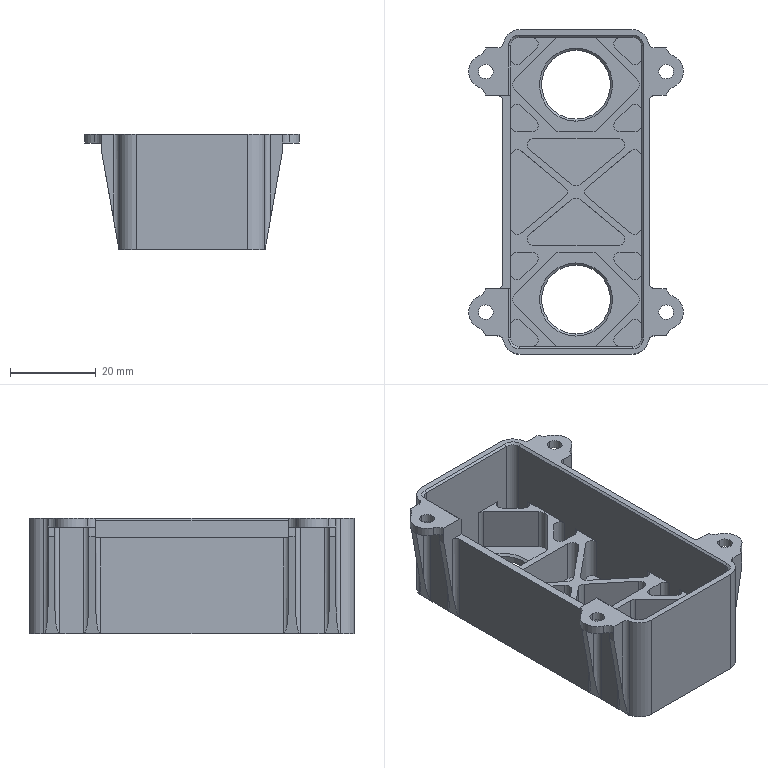NC program | NX | posted with a generic post | part box 50 x 75.58 x 26.8 mm
Lines 15469 to 16372 of 35818:
(CAVITY_MILL_COPY_COPY_COPY , TOOL : D3)
N30900 T17 M6
N30902 G54
N30904 G17 G0 G90 X-12.674 Y-33.89 S8500 M3
N30906 G43 Z30. H17
N30908 Z-13.949
N30910 G94 G1 Z-14.949 F1000.
N30912 X-12.616 Y-33.99
N30914 G3 X-11.75 Y-34.49 R1.
N30916 G1 X-10.295 F800.
N30918 X-11.324 Y-33.461
N30920 G3 X-12.29 Y-33.202 R1.
N30922 G1 X-12.401 Y-33.232
N30924 Z-13.949
N30926 G0 X-12.674 Y-33.89 Z-14.099
N30928 G1 Z-15.099 F1000.
N30930 X-12.616 Y-33.99
N30932 G3 X-11.75 Y-34.49 R1.
N30934 G1 X-10.295 F800.
N30936 X-11.324 Y-33.461
N30938 G3 X-12.29 Y-33.202 R1.
N30940 G1 X-12.401 Y-33.232
N30942 Z-14.099
N30944 G0 X-12.674 Y-33.89 Z-14.248
N30946 G1 Z-15.248 F1000.
N30948 X-12.616 Y-33.99
N30950 G3 X-11.75 Y-34.49 R1.
N30952 G1 X-10.295 F800.
N30954 X-11.324 Y-33.461
N30956 G3 X-12.29 Y-33.202 R1.
N30958 G1 X-12.401 Y-33.232
N30960 Z-14.248
N30962 G0 X-12.674 Y-33.89 Z-14.397
N30964 G1 Z-15.397 F1000.
N30966 X-12.616 Y-33.99
N30968 G3 X-11.75 Y-34.49 R1.
N30970 G1 X-10.295 F800.
N30972 X-11.324 Y-33.461
N30974 G3 X-12.29 Y-33.202 R1.
N30976 G1 X-12.401 Y-33.232
N30978 Z-14.397
N30980 G0 X-12.674 Y-33.89 Z-14.546
N30982 G1 Z-15.546 F1000.
N30984 X-12.616 Y-33.99
N30986 G3 X-11.75 Y-34.49 R1.
N30988 G1 X-10.295 F800.
N30990 X-11.324 Y-33.461
N30992 G3 X-12.29 Y-33.202 R1.
N30994 G1 X-12.401 Y-33.232
N30996 Z-14.546
N30998 G0 X-12.674 Y-33.89 Z-14.696
N31000 G1 Z-15.696 F1000.
N31002 X-12.616 Y-33.99
N31004 G3 X-11.75 Y-34.49 R1.
N31006 G1 X-10.295 F800.
N31008 X-11.324 Y-33.461
N31010 G3 X-12.29 Y-33.202 R1.
N31012 G1 X-12.401 Y-33.232
N31014 Z-14.696
N31016 G0 X-12.674 Y-33.89 Z-14.845
N31018 G1 Z-15.845 F1000.
N31020 X-12.616 Y-33.99
N31022 G3 X-11.75 Y-34.49 R1.
N31024 G1 X-10.295 F800.
N31026 X-11.324 Y-33.461
N31028 G3 X-12.29 Y-33.202 R1.
N31030 G1 X-12.401 Y-33.232
N31032 Z-14.845
N31034 G0 X-12.674 Y-33.89 Z-14.994
N31036 G1 Z-15.994 F1000.
N31038 X-12.616 Y-33.99
N31040 G3 X-11.75 Y-34.49 R1.
N31042 G1 X-10.295 F800.
N31044 X-11.324 Y-33.461
N31046 G3 X-12.29 Y-33.202 R1.
N31048 G1 X-12.401 Y-33.232
N31050 Z-14.994
N31052 G0 X-12.674 Y-33.89 Z-15.143
N31054 G1 Z-16.143 F1000.
N31056 X-12.616 Y-33.99
N31058 G3 X-11.75 Y-34.49 R1.
N31060 G1 X-10.295 F800.
N31062 X-11.324 Y-33.461
N31064 G3 X-12.29 Y-33.202 R1.
N31066 G1 X-12.401 Y-33.232
N31068 Z-15.143
N31070 G0 X-12.674 Y-33.89 Z-15.293
N31072 G1 Z-16.293 F1000.
N31074 X-12.616 Y-33.99
N31076 G3 X-11.75 Y-34.49 R1.
N31078 G1 X-10.295 F800.
N31080 X-11.324 Y-33.461
N31082 G3 X-12.29 Y-33.202 R1.
N31084 G1 X-12.401 Y-33.232
N31086 Z-15.293
N31088 G0 X-12.674 Y-33.89 Z-15.442
N31090 G1 Z-16.442 F1000.
N31092 X-12.616 Y-33.99
N31094 G3 X-11.75 Y-34.49 R1.
N31096 G1 X-10.295 F800.
N31098 X-11.324 Y-33.461
N31100 G3 X-12.29 Y-33.202 R1.
N31102 G1 X-12.401 Y-33.232
N31104 Z-15.442
N31106 G0 X-12.674 Y-33.89 Z-15.591
N31108 G1 Z-16.591 F1000.
N31110 X-12.616 Y-33.99
N31112 G3 X-11.75 Y-34.49 R1.
N31114 G1 X-10.295 F800.
N31116 X-11.324 Y-33.461
N31118 G3 X-12.29 Y-33.202 R1.
N31120 G1 X-12.401 Y-33.232
N31122 Z-15.591
N31124 G0 X-12.674 Y-33.89 Z-15.74
N31126 G1 Z-16.74 F1000.
N31128 X-12.616 Y-33.99
N31130 G3 X-11.75 Y-34.49 R1.
N31132 G1 X-10.295 F800.
N31134 X-11.324 Y-33.461
N31136 G3 X-12.29 Y-33.202 R1.
N31138 G1 X-12.401 Y-33.232
N31140 Z-15.74
N31142 G0 X-12.674 Y-33.89 Z-15.89
N31144 G1 Z-16.89 F1000.
N31146 X-12.616 Y-33.99
N31148 G3 X-11.75 Y-34.49 R1.
N31150 G1 X-10.295 F800.
N31152 X-11.324 Y-33.461
N31154 G3 X-12.29 Y-33.202 R1.
N31156 G1 X-12.401 Y-33.232
N31158 Z-15.89
N31160 G0 X-12.674 Y-33.89 Z-16.039
N31162 G1 Z-17.039 F1000.
N31164 X-12.616 Y-33.99
N31166 G3 X-11.75 Y-34.49 R1.
N31168 G1 X-10.295 F800.
N31170 X-11.324 Y-33.461
N31172 G3 X-12.29 Y-33.202 R1.
N31174 G1 X-12.401 Y-33.232
N31176 Z-16.039
N31178 G0 X-12.674 Y-33.89 Z-16.188
N31180 G1 Z-17.188 F1000.
N31182 X-12.616 Y-33.99
N31184 G3 X-11.75 Y-34.49 R1.
N31186 G1 X-10.295 F800.
N31188 X-11.324 Y-33.461
N31190 G3 X-12.29 Y-33.202 R1.
N31192 G1 X-12.401 Y-33.232
N31194 Z-16.188
N31196 G0 X-12.674 Y-33.89 Z-16.337
N31198 G1 Z-17.337 F1000.
N31200 X-12.616 Y-33.99
N31202 G3 X-11.75 Y-34.49 R1.
N31204 G1 X-10.295 F800.
N31206 X-11.324 Y-33.461
N31208 G3 X-12.29 Y-33.202 R1.
N31210 G1 X-12.401 Y-33.232
N31212 Z-16.337
N31214 G0 X-12.674 Y-33.89 Z-16.487
N31216 G1 Z-17.487 F1000.
N31218 X-12.616 Y-33.99
N31220 G3 X-11.75 Y-34.49 R1.
N31222 G1 X-10.295 F800.
N31224 X-11.324 Y-33.461
N31226 G3 X-12.29 Y-33.202 R1.
N31228 G1 X-12.401 Y-33.232
N31230 Z-16.487
N31232 G0 X-12.674 Y-33.89 Z-16.636
N31234 G1 Z-17.636 F1000.
N31236 X-12.616 Y-33.99
N31238 G3 X-11.75 Y-34.49 R1.
N31240 G1 X-10.295 F800.
N31242 X-11.324 Y-33.461
N31244 G3 X-12.29 Y-33.202 R1.
N31246 G1 X-12.401 Y-33.232
N31248 Z-16.636
N31250 G0 X-12.674 Y-33.89 Z-16.785
N31252 G1 Z-17.785 F1000.
N31254 X-12.616 Y-33.99
N31256 G3 X-11.75 Y-34.49 R1.
N31258 G1 X-10.295 F800.
N31260 X-11.324 Y-33.461
N31262 G3 X-12.29 Y-33.202 R1.
N31264 G1 X-12.401 Y-33.232
N31266 Z-16.785
N31268 G0 X-12.674 Y-33.89 Z-16.934
N31270 G1 Z-17.934 F1000.
N31272 X-12.616 Y-33.99
N31274 G3 X-11.75 Y-34.49 R1.
N31276 G1 X-10.295 F800.
N31278 X-11.324 Y-33.461
N31280 G3 X-12.29 Y-33.202 R1.
N31282 G1 X-12.401 Y-33.232
N31284 Z-16.934
N31286 G0 X-12.674 Y-33.89 Z-17.084
N31288 G1 Z-18.084 F1000.
N31290 X-12.616 Y-33.99
N31292 G3 X-11.75 Y-34.49 R1.
N31294 G1 X-10.295 F800.
N31296 X-11.324 Y-33.461
N31298 G3 X-12.29 Y-33.202 R1.
N31300 G1 X-12.401 Y-33.232
N31302 Z-17.084
N31304 G0 X-12.674 Y-33.89 Z-17.233
N31306 G1 Z-18.233 F1000.
N31308 X-12.616 Y-33.99
N31310 G3 X-11.75 Y-34.49 R1.
N31312 G1 X-10.295 F800.
N31314 X-11.324 Y-33.461
N31316 G3 X-12.29 Y-33.202 R1.
N31318 G1 X-12.401 Y-33.232
N31320 Z-17.233
N31322 G0 X-12.674 Y-33.89 Z-17.382
N31324 G1 Z-18.382 F1000.
N31326 X-12.616 Y-33.99
N31328 G3 X-11.75 Y-34.49 R1.
N31330 G1 X-10.295 F800.
N31332 X-11.324 Y-33.461
N31334 G3 X-12.29 Y-33.202 R1.
N31336 G1 X-12.401 Y-33.232
N31338 Z-17.382
N31340 G0 X-12.674 Y-33.89 Z-17.531
N31342 G1 Z-18.531 F1000.
N31344 X-12.616 Y-33.99
N31346 G3 X-11.75 Y-34.49 R1.
N31348 G1 X-10.295 F800.
N31350 X-11.324 Y-33.461
N31352 G3 X-12.29 Y-33.202 R1.
N31354 G1 X-12.401 Y-33.232
N31356 Z-17.531
N31358 G0 X-12.674 Y-33.89 Z-17.681
N31360 G1 Z-18.681 F1000.
N31362 X-12.616 Y-33.99
N31364 G3 X-11.75 Y-34.49 R1.
N31366 G1 X-10.295 F800.
N31368 X-11.324 Y-33.461
N31370 G3 X-12.29 Y-33.202 R1.
N31372 G1 X-12.401 Y-33.232
N31374 Z-17.681
N31376 G0 X-12.674 Y-33.89 Z-17.83
N31378 G1 Z-18.83 F1000.
N31380 X-12.616 Y-33.99
N31382 G3 X-11.75 Y-34.49 R1.
N31384 G1 X-10.295 F800.
N31386 X-11.324 Y-33.461
N31388 G3 X-12.29 Y-33.202 R1.
N31390 G1 X-12.401 Y-33.232
N31392 Z-17.83
N31394 G0 X-12.674 Y-33.89 Z-17.979
N31396 G1 Z-18.979 F1000.
N31398 X-12.616 Y-33.99
N31400 G3 X-11.75 Y-34.49 R1.
N31402 G1 X-10.295 F800.
N31404 X-11.324 Y-33.461
N31406 G3 X-12.29 Y-33.202 R1.
N31408 G1 X-12.401 Y-33.232
N31410 Z-17.979
N31412 G0 X-12.674 Y-33.89 Z-18.128
N31414 G1 Z-19.128 F1000.
N31416 X-12.616 Y-33.99
N31418 G3 X-11.75 Y-34.49 R1.
N31420 G1 X-10.295 F800.
N31422 X-11.324 Y-33.461
N31424 G3 X-12.29 Y-33.202 R1.
N31426 G1 X-12.401 Y-33.232
N31428 Z-18.128
N31430 G0 X-12.674 Y-33.89 Z-18.278
N31432 G1 Z-19.278 F1000.
N31434 X-12.616 Y-33.99
N31436 G3 X-11.75 Y-34.49 R1.
N31438 G1 X-10.295 F800.
N31440 X-11.324 Y-33.461
N31442 G3 X-12.29 Y-33.202 R1.
N31444 G1 X-12.401 Y-33.232
N31446 Z-18.278
N31448 G0 X-12.674 Y-33.89 Z-18.427
N31450 G1 Z-19.427 F1000.
N31452 X-12.616 Y-33.99
N31454 G3 X-11.75 Y-34.49 R1.
N31456 G1 X-10.295 F800.
N31458 X-11.324 Y-33.461
N31460 G3 X-12.29 Y-33.202 R1.
N31462 G1 X-12.401 Y-33.232
N31464 Z-18.427
N31466 G0 X-12.674 Y-33.89 Z-18.576
N31468 G1 Z-19.576 F1000.
N31470 X-12.616 Y-33.99
N31472 G3 X-11.75 Y-34.49 R1.
N31474 G1 X-10.295 F800.
N31476 X-11.324 Y-33.461
N31478 G3 X-12.29 Y-33.202 R1.
N31480 G1 X-12.401 Y-33.232
N31482 Z-18.576
N31484 G0 X-12.674 Y-33.89 Z-18.725
N31486 G1 Z-19.725 F1000.
N31488 X-12.616 Y-33.99
N31490 G3 X-11.75 Y-34.49 R1.
N31492 G1 X-10.295 F800.
N31494 X-11.324 Y-33.461
N31496 G3 X-12.29 Y-33.202 R1.
N31498 G1 X-12.401 Y-33.232
N31500 Z-18.725
N31502 G0 X-12.674 Y-33.89 Z-18.875
N31504 G1 Z-19.875 F1000.
N31506 X-12.616 Y-33.99
N31508 G3 X-11.75 Y-34.49 R1.
N31510 G1 X-10.295 F800.
N31512 X-11.324 Y-33.461
N31514 G3 X-12.29 Y-33.202 R1.
N31516 G1 X-12.401 Y-33.232
N31518 Z-18.875
N31520 G0 X-12.674 Y-33.89 Z-19.024
N31522 G1 Z-20.024 F1000.
N31524 X-12.616 Y-33.99
N31526 G3 X-11.75 Y-34.49 R1.
N31528 G1 X-10.295 F800.
N31530 X-11.324 Y-33.461
N31532 G3 X-12.29 Y-33.202 R1.
N31534 G1 X-12.401 Y-33.232
N31536 Z-19.024
N31538 G0 X-12.674 Y-33.89 Z-19.173
N31540 G1 Z-20.173 F1000.
N31542 X-12.616 Y-33.99
N31544 G3 X-11.75 Y-34.49 R1.
N31546 G1 X-10.295 F800.
N31548 X-11.324 Y-33.461
N31550 G3 X-12.29 Y-33.202 R1.
N31552 G1 X-12.401 Y-33.232
N31554 Z-19.173
N31556 G0 X-12.674 Y-33.89 Z-19.322
N31558 G1 Z-20.322 F1000.
N31560 X-12.616 Y-33.99
N31562 G3 X-11.75 Y-34.49 R1.
N31564 G1 X-10.295 F800.
N31566 X-11.324 Y-33.461
N31568 G3 X-12.29 Y-33.202 R1.
N31570 G1 X-12.401 Y-33.232
N31572 Z-19.322
N31574 G0 X-12.674 Y-33.89 Z-19.472
N31576 G1 Z-20.472 F1000.
N31578 X-12.616 Y-33.99
N31580 G3 X-11.75 Y-34.49 R1.
N31582 G1 X-10.295 F800.
N31584 X-11.324 Y-33.461
N31586 G3 X-12.29 Y-33.202 R1.
N31588 G1 X-12.401 Y-33.232
N31590 Z-19.472
N31592 G0 X-12.674 Y-33.89 Z-19.621
N31594 G1 Z-20.621 F1000.
N31596 X-12.616 Y-33.99
N31598 G3 X-11.75 Y-34.49 R1.
N31600 G1 X-10.295 F800.
N31602 X-11.324 Y-33.461
N31604 G3 X-12.29 Y-33.202 R1.
N31606 G1 X-12.401 Y-33.232
N31608 Z-19.621
N31610 G0 X-12.674 Y-33.89 Z-19.77
N31612 G1 Z-20.77 F1000.
N31614 X-12.616 Y-33.99
N31616 G3 X-11.75 Y-34.49 R1.
N31618 G1 X-10.295 F800.
N31620 X-11.324 Y-33.461
N31622 G3 X-12.29 Y-33.202 R1.
N31624 G1 X-12.401 Y-33.232
N31626 Z-19.77
N31628 G0 X-12.674 Y-33.89 Z-19.919
N31630 G1 Z-20.919 F1000.
N31632 X-12.616 Y-33.99
N31634 G3 X-11.75 Y-34.49 R1.
N31636 G1 X-10.295 F800.
N31638 X-11.324 Y-33.461
N31640 G3 X-12.29 Y-33.202 R1.
N31642 G1 X-12.401 Y-33.232
N31644 Z-19.919
N31646 G0 X-12.674 Y-33.89 Z-20.069
N31648 G1 Z-21.069 F1000.
N31650 X-12.616 Y-33.99
N31652 G3 X-11.75 Y-34.49 R1.
N31654 G1 X-10.295 F800.
N31656 X-11.324 Y-33.461
N31658 G3 X-12.29 Y-33.202 R1.
N31660 G1 X-12.401 Y-33.232
N31662 Z-20.069
N31664 G0 X-12.674 Y-33.89 Z-20.218
N31666 G1 Z-21.218 F1000.
N31668 X-12.616 Y-33.99
N31670 G3 X-11.75 Y-34.49 R1.
N31672 G1 X-10.295 F800.
N31674 X-11.324 Y-33.461
N31676 G3 X-12.29 Y-33.202 R1.
N31678 G1 X-12.401 Y-33.232
N31680 Z-20.218
N31682 G0 X-12.674 Y-33.89 Z-20.367
N31684 G1 Z-21.367 F1000.
N31686 X-12.616 Y-33.99
N31688 G3 X-11.75 Y-34.49 R1.
N31690 G1 X-10.295 F800.
N31692 X-11.324 Y-33.461
N31694 G3 X-12.29 Y-33.202 R1.
N31696 G1 X-12.401 Y-33.232
N31698 Z-20.367
N31700 G0 X-12.674 Y-33.89 Z-20.516
N31702 G1 Z-21.516 F1000.
N31704 X-12.616 Y-33.99
N31706 G3 X-11.75 Y-34.49 R1.
N31708 G1 X-10.295 F800.
N31710 X-11.324 Y-33.461
N31712 G3 X-12.29 Y-33.202 R1.
N31714 G1 X-12.401 Y-33.232
N31716 Z-20.516
N31718 G0 X-12.674 Y-33.89 Z-20.666
N31720 G1 Z-21.666 F1000.
N31722 X-12.616 Y-33.99
N31724 G3 X-11.75 Y-34.49 R1.
N31726 G1 X-10.295 F800.
N31728 X-11.324 Y-33.461
N31730 G3 X-12.29 Y-33.202 R1.
N31732 G1 X-12.401 Y-33.232
N31734 Z-20.666
N31736 G0 X-12.674 Y-33.89 Z-20.815
N31738 G1 Z-21.815 F1000.
N31740 X-12.616 Y-33.99
N31742 G3 X-11.75 Y-34.49 R1.
N31744 G1 X-10.295 F800.
N31746 X-11.324 Y-33.461
N31748 G3 X-12.29 Y-33.202 R1.
N31750 G1 X-12.401 Y-33.232
N31752 Z-20.815
N31754 G0 X-12.674 Y-33.89 Z-20.964
N31756 G1 Z-21.964 F1000.
N31758 X-12.616 Y-33.99
N31760 G3 X-11.75 Y-34.49 R1.
N31762 G1 X-10.295 F800.
N31764 X-11.324 Y-33.461
N31766 G3 X-12.29 Y-33.202 R1.
N31768 G1 X-12.401 Y-33.232
N31770 Z-20.964
N31772 G0 X-12.674 Y-33.89 Z-21.113
N31774 G1 Z-22.113 F1000.
N31776 X-12.616 Y-33.99
N31778 G3 X-11.75 Y-34.49 R1.
N31780 G1 X-10.295 F800.
N31782 X-11.324 Y-33.461
N31784 G3 X-12.29 Y-33.202 R1.
N31786 G1 X-12.401 Y-33.232
N31788 Z-21.113
N31790 G0 X-12.674 Y-33.89 Z-21.263
N31792 G1 Z-22.263 F1000.
N31794 X-12.616 Y-33.99
N31796 G3 X-11.75 Y-34.49 R1.
N31798 G1 X-10.295 F800.
N31800 X-11.324 Y-33.461
N31802 G3 X-12.29 Y-33.202 R1.
N31804 G1 X-12.401 Y-33.232
N31806 Z-21.263
N31808 G0 X-12.674 Y-33.89 Z-21.412
N31810 G1 Z-22.412 F1000.
N31812 X-12.616 Y-33.99
N31814 G3 X-11.75 Y-34.49 R1.
N31816 G1 X-10.295 F800.
N31818 X-11.324 Y-33.461
N31820 G3 X-12.29 Y-33.202 R1.
N31822 G1 X-12.401 Y-33.232
N31824 Z-21.412
N31826 G0 X-12.674 Y-33.89 Z-21.561
N31828 G1 Z-22.561 F1000.
N31830 X-12.616 Y-33.99
N31832 G3 X-11.75 Y-34.49 R1.
N31834 G1 X-10.295 F800.
N31836 X-11.324 Y-33.461
N31838 G3 X-12.29 Y-33.202 R1.
N31840 G1 X-12.401 Y-33.232
N31842 Z-21.561
N31844 G0 X-12.674 Y-33.89 Z-21.71
N31846 G1 Z-22.71 F1000.
N31848 X-12.616 Y-33.99
N31850 G3 X-11.75 Y-34.49 R1.
N31852 G1 X-10.295 F800.
N31854 X-11.324 Y-33.461
N31856 G3 X-12.29 Y-33.202 R1.
N31858 G1 X-12.401 Y-33.232
N31860 Z-21.71
N31862 G0 X-12.674 Y-33.89 Z-21.86
N31864 G1 Z-22.86 F1000.
N31866 X-12.616 Y-33.99
N31868 G3 X-11.75 Y-34.49 R1.
N31870 G1 X-10.295 F800.
N31872 X-11.324 Y-33.461
N31874 G3 X-12.29 Y-33.202 R1.
N31876 G1 X-12.401 Y-33.232
N31878 Z-21.86
N31880 G0 X-12.674 Y-33.89 Z-22.009
N31882 G1 Z-23.009 F1000.
N31884 X-12.616 Y-33.99
N31886 G3 X-11.75 Y-34.49 R1.
N31888 G1 X-10.295 F800.
N31890 X-11.324 Y-33.461
N31892 G3 X-12.29 Y-33.202 R1.
N31894 G1 X-12.401 Y-33.232
N31896 Z-22.009
N31898 G0 X-12.674 Y-33.89 Z-22.158
N31900 G1 Z-23.158 F1000.
N31902 X-12.616 Y-33.99
N31904 G3 X-11.75 Y-34.49 R1.
N31906 G1 X-10.295 F800.
N31908 X-11.324 Y-33.461
N31910 G3 X-12.29 Y-33.202 R1.
N31912 G1 X-12.401 Y-33.232
N31914 Z-22.158
N31916 G0 X-12.674 Y-33.89 Z-22.307
N31918 G1 Z-23.307 F1000.
N31920 X-12.616 Y-33.99
N31922 G3 X-11.75 Y-34.49 R1.
N31924 G1 X-10.295 F800.
N31926 X-11.324 Y-33.461
N31928 G3 X-12.29 Y-33.202 R1.
N31930 G1 X-12.401 Y-33.232
N31932 Z-22.307
N31934 G0 X-12.674 Y-33.89 Z-22.457
N31936 G1 Z-23.457 F1000.
N31938 X-12.616 Y-33.99
N31940 G3 X-11.75 Y-34.49 R1.
N31942 G1 X-10.295 F800.
N31944 X-11.324 Y-33.461
N31946 G3 X-12.29 Y-33.202 R1.
N31948 G1 X-12.401 Y-33.232
N31950 Z-22.457
N31952 G0 X-12.674 Y-33.89 Z-22.606
N31954 G1 Z-23.606 F1000.
N31956 X-12.616 Y-33.99
N31958 G3 X-11.75 Y-34.49 R1.
N31960 G1 X-10.295 F800.
N31962 X-11.324 Y-33.461
N31964 G3 X-12.29 Y-33.202 R1.
N31966 G1 X-12.401 Y-33.232
N31968 Z-22.606
N31970 G0 X-12.674 Y-33.89 Z-22.755
N31972 G1 Z-23.755 F1000.
N31974 X-12.616 Y-33.99
N31976 G3 X-11.75 Y-34.49 R1.
N31978 G1 X-10.295 F800.
N31980 X-11.324 Y-33.461
N31982 G3 X-12.29 Y-33.202 R1.
N31984 G1 X-12.401 Y-33.232
N31986 Z-22.755
N31988 G0 X-12.674 Y-33.89 Z-22.904
N31990 G1 Z-23.904 F1000.
N31992 X-12.616 Y-33.99
N31994 G3 X-11.75 Y-34.49 R1.
N31996 G1 X-10.295 F800.
N31998 X-11.324 Y-33.461
N32000 G3 X-12.29 Y-33.202 R1.
N32002 G1 X-12.401 Y-33.232
N32004 Z-22.904
N32006 G0 X-12.674 Y-33.89 Z-23.054
N32008 G1 Z-24.054 F1000.
N32010 X-12.616 Y-33.99
N32012 G3 X-11.75 Y-34.49 R1.
N32014 G1 X-10.295 F800.
N32016 X-11.324 Y-33.461
N32018 G3 X-12.29 Y-33.202 R1.
N32020 G1 X-12.401 Y-33.232
N32022 Z-23.054
N32024 G0 X-12.674 Y-33.89 Z-23.203
N32026 G1 Z-24.203 F1000.
N32028 X-12.616 Y-33.99
N32030 G3 X-11.75 Y-34.49 R1.
N32032 G1 X-10.295 F800.
N32034 X-11.324 Y-33.461
N32036 G3 X-12.29 Y-33.202 R1.
N32038 G1 X-12.401 Y-33.232
N32040 Z-23.203
N32042 G0 X-12.674 Y-33.89 Z-23.352
N32044 G1 Z-24.352 F1000.
N32046 X-12.616 Y-33.99
N32048 G3 X-11.75 Y-34.49 R1.
N32050 G1 X-10.295 F800.
N32052 X-11.324 Y-33.461
N32054 G3 X-12.29 Y-33.202 R1.
N32056 G1 X-12.401 Y-33.232
N32058 Z-23.352
N32060 G0 X-12.674 Y-33.89 Z-23.501
N32062 G1 Z-24.501 F1000.
N32064 X-12.616 Y-33.99
N32066 G3 X-11.75 Y-34.49 R1.
N32068 G1 X-10.295 F800.
N32070 X-11.324 Y-33.461
N32072 G3 X-12.29 Y-33.202 R1.
N32074 G1 X-12.401 Y-33.232
N32076 Z-23.501
N32078 G0 X-12.674 Y-33.89 Z-23.651
N32080 G1 Z-24.651 F1000.
N32082 X-12.616 Y-33.99
N32084 G3 X-11.75 Y-34.49 R1.
N32086 G1 X-10.295 F800.
N32088 X-11.324 Y-33.461
N32090 G3 X-12.29 Y-33.202 R1.
N32092 G1 X-12.401 Y-33.232
N32094 Z-23.651
N32096 G0 X-12.674 Y-33.89 Z-23.8
N32098 G1 Z-24.8 F1000.
N32100 X-12.616 Y-33.99
N32102 G3 X-11.75 Y-34.49 R1.
N32104 G1 X-10.295 F800.
N32106 X-11.324 Y-33.461
N32108 G3 X-12.29 Y-33.202 R1.
N32110 G1 X-12.401 Y-33.232
N32112 Z-23.8
N32114 G0 Z30.
N32116 X-12.442 Y-33.191
N32118 Z-13.949
N32120 G1 Z-14.949 F1000.
N32122 X-12.412 Y-33.08
N32124 G3 X-12.671 Y-32.114 R1.
N32126 G1 X-13.7 Y-31.085 F800.
N32128 Y-32.54
N32130 G3 X-13.2 Y-33.406 R1.
N32132 G1 X-13.1 Y-33.464
N32134 Z-13.949
N32136 G0 X-12.442 Y-33.191 Z-14.099
N32138 G1 Z-15.099 F1000.
N32140 X-12.412 Y-33.08
N32142 G3 X-12.671 Y-32.114 R1.
N32144 G1 X-13.7 Y-31.085 F800.
N32146 Y-32.54
N32148 G3 X-13.2 Y-33.406 R1.
N32150 G1 X-13.1 Y-33.464
N32152 Z-14.099
N32154 G0 X-12.442 Y-33.191 Z-14.248
N32156 G1 Z-15.248 F1000.
N32158 X-12.412 Y-33.08
N32160 G3 X-12.671 Y-32.114 R1.
N32162 G1 X-13.7 Y-31.085 F800.
N32164 Y-32.54
N32166 G3 X-13.2 Y-33.406 R1.
N32168 G1 X-13.1 Y-33.464
N32170 Z-14.248
N32172 G0 X-12.442 Y-33.191 Z-14.397
N32174 G1 Z-15.397 F1000.
N32176 X-12.412 Y-33.08
N32178 G3 X-12.671 Y-32.114 R1.
N32180 G1 X-13.7 Y-31.085 F800.
N32182 Y-32.54
N32184 G3 X-13.2 Y-33.406 R1.
N32186 G1 X-13.1 Y-33.464
N32188 Z-14.397
N32190 G0 X-12.442 Y-33.191 Z-14.546
N32192 G1 Z-15.546 F1000.
N32194 X-12.412 Y-33.08
N32196 G3 X-12.671 Y-32.114 R1.
N32198 G1 X-13.7 Y-31.085 F800.
N32200 Y-32.54
N32202 G3 X-13.2 Y-33.406 R1.
N32204 G1 X-13.1 Y-33.464
N32206 Z-14.546
N32208 G0 X-12.442 Y-33.191 Z-14.696
N32210 G1 Z-15.696 F1000.
N32212 X-12.412 Y-33.08
N32214 G3 X-12.671 Y-32.114 R1.
N32216 G1 X-13.7 Y-31.085 F800.
N32218 Y-32.54
N32220 G3 X-13.2 Y-33.406 R1.
N32222 G1 X-13.1 Y-33.464
N32224 Z-14.696
N32226 G0 X-12.442 Y-33.191 Z-14.845
N32228 G1 Z-15.845 F1000.
N32230 X-12.412 Y-33.08
N32232 G3 X-12.671 Y-32.114 R1.
N32234 G1 X-13.7 Y-31.085 F800.
N32236 Y-32.54
N32238 G3 X-13.2 Y-33.406 R1.
N32240 G1 X-13.1 Y-33.464
N32242 Z-14.845
N32244 G0 X-12.442 Y-33.191 Z-14.994
N32246 G1 Z-15.994 F1000.
N32248 X-12.412 Y-33.08
N32250 G3 X-12.671 Y-32.114 R1.
N32252 G1 X-13.7 Y-31.085 F800.
N32254 Y-32.54
N32256 G3 X-13.2 Y-33.406 R1.
N32258 G1 X-13.1 Y-33.464
N32260 Z-14.994
N32262 G0 X-12.442 Y-33.191 Z-15.143
N32264 G1 Z-16.143 F1000.
N32266 X-12.412 Y-33.08
N32268 G3 X-12.671 Y-32.114 R1.
N32270 G1 X-13.7 Y-31.085 F800.
N32272 Y-32.54
N32274 G3 X-13.2 Y-33.406 R1.
N32276 G1 X-13.1 Y-33.464
N32278 Z-15.143
N32280 G0 X-12.442 Y-33.191 Z-15.293
N32282 G1 Z-16.293 F1000.
N32284 X-12.412 Y-33.08
N32286 G3 X-12.671 Y-32.114 R1.
N32288 G1 X-13.7 Y-31.085 F800.
N32290 Y-32.54
N32292 G3 X-13.2 Y-33.406 R1.
N32294 G1 X-13.1 Y-33.464
N32296 Z-15.293
N32298 G0 X-12.442 Y-33.191 Z-15.442
N32300 G1 Z-16.442 F1000.
N32302 X-12.412 Y-33.08
N32304 G3 X-12.671 Y-32.114 R1.
N32306 G1 X-13.7 Y-31.085 F800.
N32308 Y-32.54
N32310 G3 X-13.2 Y-33.406 R1.
N32312 G1 X-13.1 Y-33.464
N32314 Z-15.442
N32316 G0 X-12.442 Y-33.191 Z-15.591
N32318 G1 Z-16.591 F1000.
N32320 X-12.412 Y-33.08
N32322 G3 X-12.671 Y-32.114 R1.
N32324 G1 X-13.7 Y-31.085 F800.
N32326 Y-32.54
N32328 G3 X-13.2 Y-33.406 R1.
N32330 G1 X-13.1 Y-33.464
N32332 Z-15.591
N32334 G0 X-12.442 Y-33.191 Z-15.74
N32336 G1 Z-16.74 F1000.
N32338 X-12.412 Y-33.08
N32340 G3 X-12.671 Y-32.114 R1.
N32342 G1 X-13.7 Y-31.085 F800.
N32344 Y-32.54
N32346 G3 X-13.2 Y-33.406 R1.
N32348 G1 X-13.1 Y-33.464
N32350 Z-15.74
N32352 G0 X-12.442 Y-33.191 Z-15.89
N32354 G1 Z-16.89 F1000.
N32356 X-12.412 Y-33.08
N32358 G3 X-12.671 Y-32.114 R1.
N32360 G1 X-13.7 Y-31.085 F800.
N32362 Y-32.54
N32364 G3 X-13.2 Y-33.406 R1.
N32366 G1 X-13.1 Y-33.464
N32368 Z-15.89
N32370 G0 X-12.442 Y-33.191 Z-16.039
N32372 G1 Z-17.039 F1000.
N32374 X-12.412 Y-33.08
N32376 G3 X-12.671 Y-32.114 R1.
N32378 G1 X-13.7 Y-31.085 F800.
N32380 Y-32.54
N32382 G3 X-13.2 Y-33.406 R1.
N32384 G1 X-13.1 Y-33.464
N32386 Z-16.039
N32388 G0 X-12.442 Y-33.191 Z-16.188
N32390 G1 Z-17.188 F1000.
N32392 X-12.412 Y-33.08
N32394 G3 X-12.671 Y-32.114 R1.
N32396 G1 X-13.7 Y-31.085 F800.
N32398 Y-32.54
N32400 G3 X-13.2 Y-33.406 R1.
N32402 G1 X-13.1 Y-33.464
N32404 Z-16.188
N32406 G0 X-12.442 Y-33.191 Z-16.337
N32408 G1 Z-17.337 F1000.
N32410 X-12.412 Y-33.08
N32412 G3 X-12.671 Y-32.114 R1.
N32414 G1 X-13.7 Y-31.085 F800.
N32416 Y-32.54
N32418 G3 X-13.2 Y-33.406 R1.
N32420 G1 X-13.1 Y-33.464
N32422 Z-16.337
N32424 G0 X-12.442 Y-33.191 Z-16.487
N32426 G1 Z-17.487 F1000.
N32428 X-12.412 Y-33.08
N32430 G3 X-12.671 Y-32.114 R1.
N32432 G1 X-13.7 Y-31.085 F800.
N32434 Y-32.54
N32436 G3 X-13.2 Y-33.406 R1.
N32438 G1 X-13.1 Y-33.464
N32440 Z-16.487
N32442 G0 X-12.442 Y-33.191 Z-16.636
N32444 G1 Z-17.636 F1000.
N32446 X-12.412 Y-33.08
N32448 G3 X-12.671 Y-32.114 R1.
N32450 G1 X-13.7 Y-31.085 F800.
N32452 Y-32.54
N32454 G3 X-13.2 Y-33.406 R1.
N32456 G1 X-13.1 Y-33.464
N32458 Z-16.636
N32460 G0 X-12.442 Y-33.191 Z-16.785
N32462 G1 Z-17.785 F1000.
N32464 X-12.412 Y-33.08
N32466 G3 X-12.671 Y-32.114 R1.
N32468 G1 X-13.7 Y-31.085 F800.
N32470 Y-32.54
N32472 G3 X-13.2 Y-33.406 R1.
N32474 G1 X-13.1 Y-33.464
N32476 Z-16.785
N32478 G0 X-12.442 Y-33.191 Z-16.934
N32480 G1 Z-17.934 F1000.
N32482 X-12.412 Y-33.08
N32484 G3 X-12.671 Y-32.114 R1.
N32486 G1 X-13.7 Y-31.085 F800.
N32488 Y-32.54
N32490 G3 X-13.2 Y-33.406 R1.
N32492 G1 X-13.1 Y-33.464
N32494 Z-16.934
N32496 G0 X-12.442 Y-33.191 Z-17.084
N32498 G1 Z-18.084 F1000.
N32500 X-12.412 Y-33.08
N32502 G3 X-12.671 Y-32.114 R1.
N32504 G1 X-13.7 Y-31.085 F800.
N32506 Y-32.54
N32508 G3 X-13.2 Y-33.406 R1.
N32510 G1 X-13.1 Y-33.464
N32512 Z-17.084
N32514 G0 X-12.442 Y-33.191 Z-17.233
N32516 G1 Z-18.233 F1000.
N32518 X-12.412 Y-33.08
N32520 G3 X-12.671 Y-32.114 R1.
N32522 G1 X-13.7 Y-31.085 F800.
N32524 Y-32.54
N32526 G3 X-13.2 Y-33.406 R1.
N32528 G1 X-13.1 Y-33.464
N32530 Z-17.233
N32532 G0 X-12.442 Y-33.191 Z-17.382
N32534 G1 Z-18.382 F1000.
N32536 X-12.412 Y-33.08
N32538 G3 X-12.671 Y-32.114 R1.
N32540 G1 X-13.7 Y-31.085 F800.
N32542 Y-32.54
N32544 G3 X-13.2 Y-33.406 R1.
N32546 G1 X-13.1 Y-33.464
N32548 Z-17.382
N32550 G0 X-12.442 Y-33.191 Z-17.531
N32552 G1 Z-18.531 F1000.
N32554 X-12.412 Y-33.08
N32556 G3 X-12.671 Y-32.114 R1.
N32558 G1 X-13.7 Y-31.085 F800.
N32560 Y-32.54
N32562 G3 X-13.2 Y-33.406 R1.
N32564 G1 X-13.1 Y-33.464
N32566 Z-17.531
N32568 G0 X-12.442 Y-33.191 Z-17.681
N32570 G1 Z-18.681 F1000.
N32572 X-12.412 Y-33.08
N32574 G3 X-12.671 Y-32.114 R1.
N32576 G1 X-13.7 Y-31.085 F800.
N32578 Y-32.54
N32580 G3 X-13.2 Y-33.406 R1.
N32582 G1 X-13.1 Y-33.464
N32584 Z-17.681
N32586 G0 X-12.442 Y-33.191 Z-17.83
N32588 G1 Z-18.83 F1000.
N32590 X-12.412 Y-33.08
N32592 G3 X-12.671 Y-32.114 R1.
N32594 G1 X-13.7 Y-31.085 F800.
N32596 Y-32.54
N32598 G3 X-13.2 Y-33.406 R1.
N32600 G1 X-13.1 Y-33.464
N32602 Z-17.83
N32604 G0 X-12.442 Y-33.191 Z-17.979
N32606 G1 Z-18.979 F1000.
N32608 X-12.412 Y-33.08
N32610 G3 X-12.671 Y-32.114 R1.
N32612 G1 X-13.7 Y-31.085 F800.
N32614 Y-32.54
N32616 G3 X-13.2 Y-33.406 R1.
N32618 G1 X-13.1 Y-33.464
N32620 Z-17.979
N32622 G0 X-12.442 Y-33.191 Z-18.128
N32624 G1 Z-19.128 F1000.
N32626 X-12.412 Y-33.08
N32628 G3 X-12.671 Y-32.114 R1.
N32630 G1 X-13.7 Y-31.085 F800.
N32632 Y-32.54
N32634 G3 X-13.2 Y-33.406 R1.
N32636 G1 X-13.1 Y-33.464
N32638 Z-18.128
N32640 G0 X-12.442 Y-33.191 Z-18.278
N32642 G1 Z-19.278 F1000.
N32644 X-12.412 Y-33.08
N32646 G3 X-12.671 Y-32.114 R1.
N32648 G1 X-13.7 Y-31.085 F800.
N32650 Y-32.54
N32652 G3 X-13.2 Y-33.406 R1.
N32654 G1 X-13.1 Y-33.464
N32656 Z-18.278
N32658 G0 X-12.442 Y-33.191 Z-18.427
N32660 G1 Z-19.427 F1000.
N32662 X-12.412 Y-33.08
N32664 G3 X-12.671 Y-32.114 R1.
N32666 G1 X-13.7 Y-31.085 F800.
N32668 Y-32.54
N32670 G3 X-13.2 Y-33.406 R1.
N32672 G1 X-13.1 Y-33.464
N32674 Z-18.427
N32676 G0 X-12.442 Y-33.191 Z-18.576
N32678 G1 Z-19.576 F1000.
N32680 X-12.412 Y-33.08
N32682 G3 X-12.671 Y-32.114 R1.
N32684 G1 X-13.7 Y-31.085 F800.
N32686 Y-32.54
N32688 G3 X-13.2 Y-33.406 R1.
N32690 G1 X-13.1 Y-33.464
N32692 Z-18.576
N32694 G0 X-12.442 Y-33.191 Z-18.725
N32696 G1 Z-19.725 F1000.
N32698 X-12.412 Y-33.08
N32700 G3 X-12.671 Y-32.114 R1.